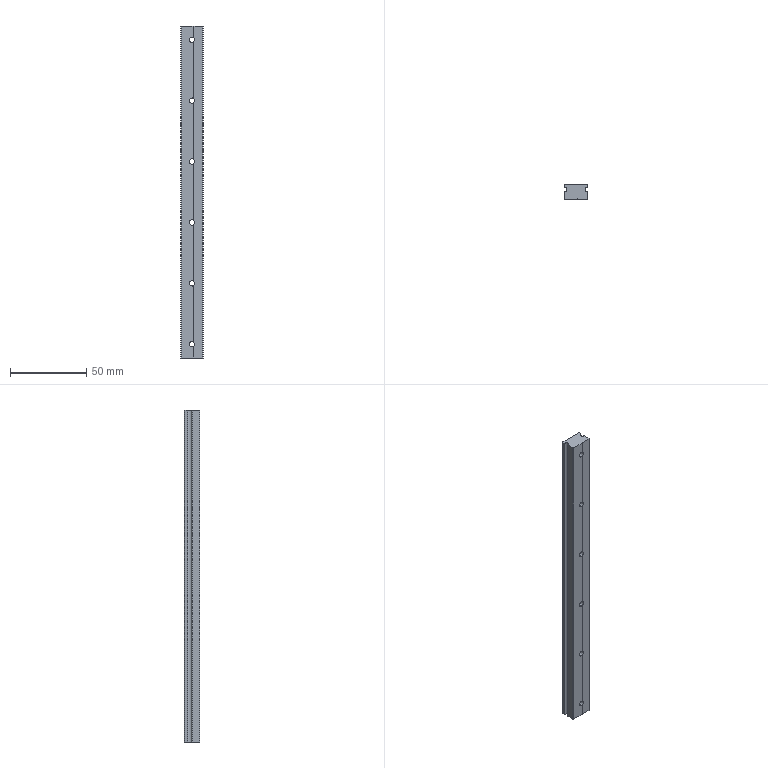Part | STEP file | 11-MANIFOLD_SOLID_BREP_4011 | 1 solid | 53 faces | box 15 x 10 x 218 mm | volume 29980 mm3 | cylinder 34 | plane 19 | commonest cylinder face diameters 3.5 x12 6 x12 0.6 x7 3 x3